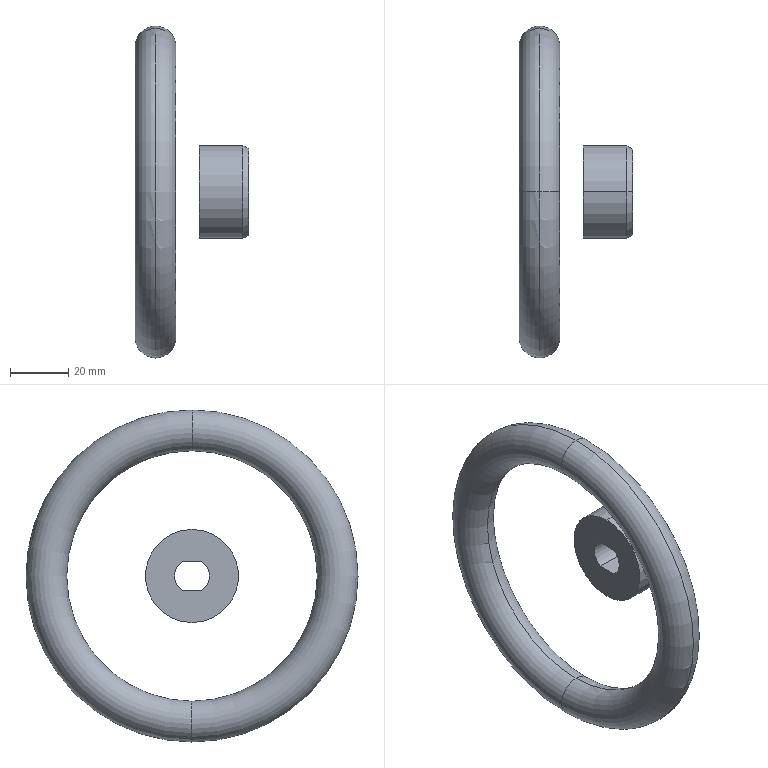Part | SolidWorks | features ICE 2, Chamfer 1, Sweep 1 | 2 solids | 14 faces | box 39 x 114 x 114 mm | volume 60150 mm3 | torus 4 | cylinder 4 | plane 4 | cone 2 | commonest cylinder face diameters 12 x2 32 x2
STEP:
#1=CARTESIAN_POINT('',(0.,-50.,-57.));
#2=VERTEX_POINT('',#1);
#3=CARTESIAN_POINT('',(0.,-50.,-43.));
#4=VERTEX_POINT('',#3);
#5=CARTESIAN_POINT('',(0.,-50.,-50.));
#6=DIRECTION('',(0.,1.,0.));
#7=DIRECTION('',(0.,0.,1.));
#8=AXIS2_PLACEMENT_3D('',#5,#6,#7);
#9=CIRCLE('',#8,7.);
#10=EDGE_CURVE('',#2,#4,#9,.T.);
#11=ORIENTED_EDGE('',*,*,#10,.F.);
#12=CARTESIAN_POINT('',(0.,-50.,57.));
#13=VERTEX_POINT('',#12);
#14=CARTESIAN_POINT('',(0.,-50.,0.));
#15=DIRECTION('',(-1.,0.,0.));
#16=DIRECTION('',(0.,0.,1.));
#17=AXIS2_PLACEMENT_3D('',#14,#15,#16);
#18=CIRCLE('',#17,57.);
#19=EDGE_CURVE('',#2,#13,#18,.T.);
#20=ORIENTED_EDGE('',*,*,#19,.T.);
#21=CARTESIAN_POINT('',(0.,-50.,43.));
#22=VERTEX_POINT('',#21);
#23=CARTESIAN_POINT('',(0.,-50.,50.));
#24=DIRECTION('',(0.,-1.,0.));
#25=DIRECTION('',(0.,0.,-1.));
#26=AXIS2_PLACEMENT_3D('',#23,#24,#25);
#27=CIRCLE('',#26,7.);
#28=EDGE_CURVE('',#13,#22,#27,.T.);
#29=ORIENTED_EDGE('',*,*,#28,.T.);
#30=CARTESIAN_POINT('',(0.,-50.,0.));
#31=DIRECTION('',(-1.,0.,0.));
#32=DIRECTION('',(0.,0.,1.));
#33=AXIS2_PLACEMENT_3D('',#30,#31,#32);
#34=CIRCLE('',#33,43.);
#35=EDGE_CURVE('',#4,#22,#34,.T.);
#36=ORIENTED_EDGE('',*,*,#35,.F.);
#37=EDGE_LOOP('',(#11,#20,#29,#36));
#38=FACE_OUTER_BOUND('',#37,.T.);
#39=CARTESIAN_POINT('',(0.,-50.,0.));
#40=DIRECTION('',(-1.,0.,0.));
#41=DIRECTION('',(0.,0.,1.));
#42=AXIS2_PLACEMENT_3D('',#39,#40,#41);
#43=TOROIDAL_SURFACE('',#42,50.,7.);
#44=ADVANCED_FACE('',(#38),#43,.T.);
#45=ORIENTED_EDGE('',*,*,#28,.F.);
#46=CARTESIAN_POINT('',(0.,-50.,0.));
#47=DIRECTION('',(-1.,0.,0.));
#48=DIRECTION('',(0.,0.,1.));
#49=AXIS2_PLACEMENT_3D('',#46,#47,#48);
#50=CIRCLE('',#49,57.);
#51=EDGE_CURVE('',#13,#2,#50,.T.);
#52=ORIENTED_EDGE('',*,*,#51,.T.);
#53=ORIENTED_EDGE('',*,*,#10,.T.);
#54=CARTESIAN_POINT('',(0.,-50.,0.));
#55=DIRECTION('',(-1.,0.,0.));
#56=DIRECTION('',(0.,0.,1.));
#57=AXIS2_PLACEMENT_3D('',#54,#55,#56);
#58=CIRCLE('',#57,43.);
#59=EDGE_CURVE('',#22,#4,#58,.T.);
#60=ORIENTED_EDGE('',*,*,#59,.F.);
#61=EDGE_LOOP('',(#45,#52,#53,#60));
#62=FACE_OUTER_BOUND('',#61,.T.);
#63=CARTESIAN_POINT('',(0.,-50.,0.));
#64=DIRECTION('',(-1.,0.,0.));
#65=DIRECTION('',(0.,0.,1.));
#66=AXIS2_PLACEMENT_3D('',#63,#64,#65);
#67=TOROIDAL_SURFACE('',#66,50.,7.);
#68=ADVANCED_FACE('',(#62),#67,.T.);
#69=ORIENTED_EDGE('',*,*,#51,.F.);
#70=CARTESIAN_POINT('',(0.,-50.,50.));
#71=DIRECTION('',(0.,-1.,0.));
#72=DIRECTION('',(0.,0.,-1.));
#73=AXIS2_PLACEMENT_3D('',#70,#71,#72);
#74=CIRCLE('',#73,7.);
#75=EDGE_CURVE('',#22,#13,#74,.T.);
#76=ORIENTED_EDGE('',*,*,#75,.F.);
#77=ORIENTED_EDGE('',*,*,#59,.T.);
#78=CARTESIAN_POINT('',(0.,-50.,-50.));
#79=DIRECTION('',(0.,1.,0.));
#80=DIRECTION('',(0.,0.,1.));
#81=AXIS2_PLACEMENT_3D('',#78,#79,#80);
#82=CIRCLE('',#81,7.);
#83=EDGE_CURVE('',#4,#2,#82,.T.);
#84=ORIENTED_EDGE('',*,*,#83,.T.);
#85=EDGE_LOOP('',(#69,#76,#77,#84));
#86=FACE_OUTER_BOUND('',#85,.T.);
#87=CARTESIAN_POINT('',(0.,-50.,0.));
#88=DIRECTION('',(-1.,0.,0.));
#89=DIRECTION('',(0.,0.,1.));
#90=AXIS2_PLACEMENT_3D('',#87,#88,#89);
#91=TOROIDAL_SURFACE('',#90,50.,7.);
#92=ADVANCED_FACE('',(#86),#91,.T.);
#93=ORIENTED_EDGE('',*,*,#19,.F.);
#94=ORIENTED_EDGE('',*,*,#83,.F.);
#95=ORIENTED_EDGE('',*,*,#35,.T.);
#96=ORIENTED_EDGE('',*,*,#75,.T.);
#97=EDGE_LOOP('',(#93,#94,#95,#96));
#98=FACE_OUTER_BOUND('',#97,.T.);
#99=CARTESIAN_POINT('',(0.,-50.,0.));
#100=DIRECTION('',(-1.,0.,0.));
#101=DIRECTION('',(0.,0.,1.));
#102=AXIS2_PLACEMENT_3D('',#99,#100,#101);
#103=TOROIDAL_SURFACE('',#102,50.,7.);
#104=ADVANCED_FACE('',(#98),#103,.T.);
#105=CLOSED_SHELL('',(#44,#68,#92,#104));
#106=MANIFOLD_SOLID_BREP('',#105);
#107=CARTESIAN_POINT('',(32.,-50.,-14.845));
#108=VERTEX_POINT('',#107);
#109=CARTESIAN_POINT('',(32.,-50.,14.845));
#110=VERTEX_POINT('',#109);
#111=CARTESIAN_POINT('',(32.,-50.,0.));
#112=DIRECTION('',(1.,0.,0.));
#113=DIRECTION('',(0.,0.,-1.));
#114=AXIS2_PLACEMENT_3D('',#111,#112,#113);
#115=CIRCLE('',#114,14.845);
#116=EDGE_CURVE('',#108,#110,#115,.T.);
#117=ORIENTED_EDGE('',*,*,#116,.F.);
#118=CARTESIAN_POINT('',(30.,-50.,-16.));
#119=VERTEX_POINT('',#118);
#120=CARTESIAN_POINT('',(32.,-50.,-14.845));
#121=DIRECTION('',(-0.866,0.,-0.5));
#122=VECTOR('',#121,1000.);
#123=LINE('',#120,#122);
#124=EDGE_CURVE('',#108,#119,#123,.T.);
#125=ORIENTED_EDGE('',*,*,#124,.T.);
#126=CARTESIAN_POINT('',(30.,-50.,16.));
#127=VERTEX_POINT('',#126);
#128=CARTESIAN_POINT('',(30.,-50.,0.));
#129=DIRECTION('',(-1.,0.,0.));
#130=DIRECTION('',(0.,0.,-1.));
#131=AXIS2_PLACEMENT_3D('',#128,#129,#130);
#132=CIRCLE('',#131,16.);
#133=EDGE_CURVE('',#127,#119,#132,.T.);
#134=ORIENTED_EDGE('',*,*,#133,.F.);
#135=CARTESIAN_POINT('',(32.,-50.,14.845));
#136=DIRECTION('',(-0.866,0.,0.5));
#137=VECTOR('',#136,1000.);
#138=LINE('',#135,#137);
#139=EDGE_CURVE('',#110,#127,#138,.T.);
#140=ORIENTED_EDGE('',*,*,#139,.F.);
#141=EDGE_LOOP('',(#117,#125,#134,#140));
#142=FACE_OUTER_BOUND('',#141,.T.);
#143=CARTESIAN_POINT('',(32.,-50.,0.));
#144=DIRECTION('',(-1.,0.,0.));
#145=DIRECTION('',(0.,0.,1.));
#146=AXIS2_PLACEMENT_3D('',#143,#144,#145);
#147=CONICAL_SURFACE('',#146,14.845,0.5236);
#148=ADVANCED_FACE('',(#142),#147,.T.);
#149=CARTESIAN_POINT('',(15.,-50.,-16.));
#150=VERTEX_POINT('',#149);
#151=CARTESIAN_POINT('',(15.,-50.,16.));
#152=VERTEX_POINT('',#151);
#153=CARTESIAN_POINT('',(15.,-50.,0.));
#154=DIRECTION('',(1.,0.,0.));
#155=DIRECTION('',(0.,0.,-1.));
#156=AXIS2_PLACEMENT_3D('',#153,#154,#155);
#157=CIRCLE('',#156,16.);
#158=EDGE_CURVE('',#150,#152,#157,.T.);
#159=ORIENTED_EDGE('',*,*,#158,.T.);
#160=CARTESIAN_POINT('',(15.,-50.,16.));
#161=DIRECTION('',(1.,0.,0.));
#162=VECTOR('',#161,1000.);
#163=LINE('',#160,#162);
#164=EDGE_CURVE('',#152,#127,#163,.T.);
#165=ORIENTED_EDGE('',*,*,#164,.T.);
#166=ORIENTED_EDGE('',*,*,#133,.T.);
#167=CARTESIAN_POINT('',(15.,-50.,-16.));
#168=DIRECTION('',(1.,0.,0.));
#169=VECTOR('',#168,1000.);
#170=LINE('',#167,#169);
#171=EDGE_CURVE('',#150,#119,#170,.T.);
#172=ORIENTED_EDGE('',*,*,#171,.F.);
#173=EDGE_LOOP('',(#159,#165,#166,#172));
#174=FACE_OUTER_BOUND('',#173,.T.);
#175=CARTESIAN_POINT('',(15.,-50.,0.));
#176=DIRECTION('',(1.,0.,0.));
#177=DIRECTION('',(0.,0.,-1.));
#178=AXIS2_PLACEMENT_3D('',#175,#176,#177);
#179=CYLINDRICAL_SURFACE('',#178,16.);
#180=ADVANCED_FACE('',(#174),#179,.T.);
#181=ORIENTED_EDGE('',*,*,#164,.F.);
#182=CARTESIAN_POINT('',(15.,-50.,0.));
#183=DIRECTION('',(1.,0.,0.));
#184=DIRECTION('',(0.,0.,-1.));
#185=AXIS2_PLACEMENT_3D('',#182,#183,#184);
#186=CIRCLE('',#185,16.);
#187=EDGE_CURVE('',#152,#150,#186,.T.);
#188=ORIENTED_EDGE('',*,*,#187,.T.);
#189=ORIENTED_EDGE('',*,*,#171,.T.);
#190=CARTESIAN_POINT('',(30.,-50.,0.));
#191=DIRECTION('',(-1.,0.,0.));
#192=DIRECTION('',(0.,0.,-1.));
#193=AXIS2_PLACEMENT_3D('',#190,#191,#192);
#194=CIRCLE('',#193,16.);
#195=EDGE_CURVE('',#119,#127,#194,.T.);
#196=ORIENTED_EDGE('',*,*,#195,.T.);
#197=EDGE_LOOP('',(#181,#188,#189,#196));
#198=FACE_OUTER_BOUND('',#197,.T.);
#199=CARTESIAN_POINT('',(15.,-50.,0.));
#200=DIRECTION('',(1.,0.,0.));
#201=DIRECTION('',(0.,0.,-1.));
#202=AXIS2_PLACEMENT_3D('',#199,#200,#201);
#203=CYLINDRICAL_SURFACE('',#202,16.);
#204=ADVANCED_FACE('',(#198),#203,.T.);
#205=CARTESIAN_POINT('',(15.,-53.317,-5.));
#206=VERTEX_POINT('',#205);
#207=CARTESIAN_POINT('',(15.,-46.683,-5.));
#208=VERTEX_POINT('',#207);
#209=CARTESIAN_POINT('',(15.,-50.,-5.));
#210=DIRECTION('',(0.,1.,0.));
#211=VECTOR('',#210,1000.);
#212=LINE('',#209,#211);
#213=EDGE_CURVE('',#206,#208,#212,.T.);
#214=ORIENTED_EDGE('',*,*,#213,.T.);
#215=CARTESIAN_POINT('',(15.,-46.683,5.));
#216=VERTEX_POINT('',#215);
#217=CARTESIAN_POINT('',(15.,-50.,0.));
#218=DIRECTION('',(1.,0.,0.));
#219=DIRECTION('',(0.,0.,-1.));
#220=AXIS2_PLACEMENT_3D('',#217,#218,#219);
#221=CIRCLE('',#220,6.);
#222=EDGE_CURVE('',#208,#216,#221,.T.);
#223=ORIENTED_EDGE('',*,*,#222,.T.);
#224=CARTESIAN_POINT('',(15.,-53.317,5.));
#225=VERTEX_POINT('',#224);
#226=CARTESIAN_POINT('',(15.,-50.,5.));
#227=DIRECTION('',(0.,-1.,0.));
#228=VECTOR('',#227,1000.);
#229=LINE('',#226,#228);
#230=EDGE_CURVE('',#216,#225,#229,.T.);
#231=ORIENTED_EDGE('',*,*,#230,.T.);
#232=CARTESIAN_POINT('',(15.,-50.,0.));
#233=DIRECTION('',(1.,0.,0.));
#234=DIRECTION('',(0.,0.,-1.));
#235=AXIS2_PLACEMENT_3D('',#232,#233,#234);
#236=CIRCLE('',#235,6.);
#237=EDGE_CURVE('',#225,#206,#236,.T.);
#238=ORIENTED_EDGE('',*,*,#237,.T.);
#239=EDGE_LOOP('',(#214,#223,#231,#238));
#240=FACE_BOUND('',#239,.T.);
#241=ORIENTED_EDGE('',*,*,#158,.F.);
#242=ORIENTED_EDGE('',*,*,#187,.F.);
#243=EDGE_LOOP('',(#241,#242));
#244=FACE_OUTER_BOUND('',#243,.T.);
#245=CARTESIAN_POINT('',(15.,-50.,0.));
#246=DIRECTION('',(1.,0.,0.));
#247=DIRECTION('',(0.,0.,-1.));
#248=AXIS2_PLACEMENT_3D('',#245,#246,#247);
#249=PLANE('',#248);
#250=ADVANCED_FACE('',(#240,#244),#249,.F.);
#251=CARTESIAN_POINT('',(32.,-46.683,-5.));
#252=VERTEX_POINT('',#251);
#253=CARTESIAN_POINT('',(32.,-46.683,5.));
#254=VERTEX_POINT('',#253);
#255=CARTESIAN_POINT('',(32.,-50.,0.));
#256=DIRECTION('',(1.,0.,0.));
#257=DIRECTION('',(0.,0.,-1.));
#258=AXIS2_PLACEMENT_3D('',#255,#256,#257);
#259=CIRCLE('',#258,6.);
#260=EDGE_CURVE('',#252,#254,#259,.T.);
#261=ORIENTED_EDGE('',*,*,#260,.F.);
#262=CARTESIAN_POINT('',(32.,-53.317,-5.));
#263=VERTEX_POINT('',#262);
#264=CARTESIAN_POINT('',(32.,-46.683,-5.));
#265=DIRECTION('',(0.,1.,0.));
#266=VECTOR('',#265,1000.);
#267=LINE('',#264,#266);
#268=EDGE_CURVE('',#263,#252,#267,.T.);
#269=ORIENTED_EDGE('',*,*,#268,.F.);
#270=CARTESIAN_POINT('',(32.,-53.317,5.));
#271=VERTEX_POINT('',#270);
#272=CARTESIAN_POINT('',(32.,-50.,0.));
#273=DIRECTION('',(1.,0.,0.));
#274=DIRECTION('',(0.,0.,-1.));
#275=AXIS2_PLACEMENT_3D('',#272,#273,#274);
#276=CIRCLE('',#275,6.);
#277=EDGE_CURVE('',#271,#263,#276,.T.);
#278=ORIENTED_EDGE('',*,*,#277,.F.);
#279=CARTESIAN_POINT('',(32.,-46.683,5.));
#280=DIRECTION('',(0.,-1.,0.));
#281=VECTOR('',#280,1000.);
#282=LINE('',#279,#281);
#283=EDGE_CURVE('',#254,#271,#282,.T.);
#284=ORIENTED_EDGE('',*,*,#283,.F.);
#285=EDGE_LOOP('',(#261,#269,#278,#284));
#286=FACE_BOUND('',#285,.T.);
#287=CARTESIAN_POINT('',(32.,-50.,0.));
#288=DIRECTION('',(1.,0.,0.));
#289=DIRECTION('',(0.,0.,-1.));
#290=AXIS2_PLACEMENT_3D('',#287,#288,#289);
#291=CIRCLE('',#290,14.845);
#292=EDGE_CURVE('',#110,#108,#291,.T.);
#293=ORIENTED_EDGE('',*,*,#292,.T.);
#294=ORIENTED_EDGE('',*,*,#116,.T.);
#295=EDGE_LOOP('',(#293,#294));
#296=FACE_OUTER_BOUND('',#295,.T.);
#297=CARTESIAN_POINT('',(32.,-50.,0.));
#298=DIRECTION('',(1.,0.,0.));
#299=DIRECTION('',(0.,0.,-1.));
#300=AXIS2_PLACEMENT_3D('',#297,#298,#299);
#301=PLANE('',#300);
#302=ADVANCED_FACE('',(#286,#296),#301,.T.);
#303=ORIENTED_EDGE('',*,*,#124,.F.);
#304=ORIENTED_EDGE('',*,*,#292,.F.);
#305=ORIENTED_EDGE('',*,*,#139,.T.);
#306=ORIENTED_EDGE('',*,*,#195,.F.);
#307=EDGE_LOOP('',(#303,#304,#305,#306));
#308=FACE_OUTER_BOUND('',#307,.T.);
#309=CARTESIAN_POINT('',(32.,-50.,0.));
#310=DIRECTION('',(-1.,0.,0.));
#311=DIRECTION('',(0.,0.,1.));
#312=AXIS2_PLACEMENT_3D('',#309,#310,#311);
#313=CONICAL_SURFACE('',#312,14.845,0.5236);
#314=ADVANCED_FACE('',(#308),#313,.T.);
#315=CARTESIAN_POINT('',(-7.,-46.683,-5.));
#316=DIRECTION('',(1.,0.,0.));
#317=VECTOR('',#316,1000.);
#318=LINE('',#315,#317);
#319=EDGE_CURVE('',#208,#252,#318,.T.);
#320=ORIENTED_EDGE('',*,*,#319,.T.);
#321=ORIENTED_EDGE('',*,*,#260,.T.);
#322=CARTESIAN_POINT('',(-7.,-46.683,5.));
#323=DIRECTION('',(1.,0.,0.));
#324=VECTOR('',#323,1000.);
#325=LINE('',#322,#324);
#326=EDGE_CURVE('',#216,#254,#325,.T.);
#327=ORIENTED_EDGE('',*,*,#326,.F.);
#328=ORIENTED_EDGE('',*,*,#222,.F.);
#329=EDGE_LOOP('',(#320,#321,#327,#328));
#330=FACE_OUTER_BOUND('',#329,.T.);
#331=CARTESIAN_POINT('',(-7.,-50.,0.));
#332=DIRECTION('',(1.,0.,0.));
#333=DIRECTION('',(0.,0.,-1.));
#334=AXIS2_PLACEMENT_3D('',#331,#332,#333);
#335=CYLINDRICAL_SURFACE('',#334,6.);
#336=ADVANCED_FACE('',(#330),#335,.F.);
#337=CARTESIAN_POINT('',(-7.,-53.317,-5.));
#338=DIRECTION('',(1.,0.,0.));
#339=VECTOR('',#338,1000.);
#340=LINE('',#337,#339);
#341=EDGE_CURVE('',#206,#263,#340,.T.);
#342=ORIENTED_EDGE('',*,*,#341,.T.);
#343=ORIENTED_EDGE('',*,*,#268,.T.);
#344=ORIENTED_EDGE('',*,*,#319,.F.);
#345=ORIENTED_EDGE('',*,*,#213,.F.);
#346=EDGE_LOOP('',(#342,#343,#344,#345));
#347=FACE_OUTER_BOUND('',#346,.T.);
#348=CARTESIAN_POINT('',(-7.,-46.683,-5.));
#349=DIRECTION('',(0.,0.,-1.));
#350=DIRECTION('',(-1.,0.,0.));
#351=AXIS2_PLACEMENT_3D('',#348,#349,#350);
#352=PLANE('',#351);
#353=ADVANCED_FACE('',(#347),#352,.F.);
#354=CARTESIAN_POINT('',(-7.,-53.317,5.));
#355=DIRECTION('',(1.,0.,0.));
#356=VECTOR('',#355,1000.);
#357=LINE('',#354,#356);
#358=EDGE_CURVE('',#225,#271,#357,.T.);
#359=ORIENTED_EDGE('',*,*,#358,.T.);
#360=ORIENTED_EDGE('',*,*,#277,.T.);
#361=ORIENTED_EDGE('',*,*,#341,.F.);
#362=ORIENTED_EDGE('',*,*,#237,.F.);
#363=EDGE_LOOP('',(#359,#360,#361,#362));
#364=FACE_OUTER_BOUND('',#363,.T.);
#365=CARTESIAN_POINT('',(-7.,-50.,0.));
#366=DIRECTION('',(1.,0.,0.));
#367=DIRECTION('',(0.,0.,-1.));
#368=AXIS2_PLACEMENT_3D('',#365,#366,#367);
#369=CYLINDRICAL_SURFACE('',#368,6.);
#370=ADVANCED_FACE('',(#364),#369,.F.);
#371=ORIENTED_EDGE('',*,*,#326,.T.);
#372=ORIENTED_EDGE('',*,*,#283,.T.);
#373=ORIENTED_EDGE('',*,*,#358,.F.);
#374=ORIENTED_EDGE('',*,*,#230,.F.);
#375=EDGE_LOOP('',(#371,#372,#373,#374));
#376=FACE_OUTER_BOUND('',#375,.T.);
#377=CARTESIAN_POINT('',(-7.,-46.683,5.));
#378=DIRECTION('',(0.,0.,1.));
#379=DIRECTION('',(1.,0.,0.));
#380=AXIS2_PLACEMENT_3D('',#377,#378,#379);
#381=PLANE('',#380);
#382=ADVANCED_FACE('',(#376),#381,.F.);
#383=CLOSED_SHELL('',(#148,#180,#204,#250,#302,#314,#336,#353,#370,#382));
#384=MANIFOLD_SOLID_BREP('',#383);
#385=CARTESIAN_POINT('',(0.,0.,0.));
#386=DIRECTION('',(0.,0.,1.));
#387=DIRECTION('',(1.,0.,0.));
#388=AXIS2_PLACEMENT_3D('',#385,#386,#387);
#389=(LENGTH_UNIT()NAMED_UNIT(*)SI_UNIT(.MILLI.,.METRE.));
#390=UNCERTAINTY_MEASURE_WITH_UNIT(LENGTH_MEASURE(0.00001),#389,'','');
#391=(NAMED_UNIT(*)PLANE_ANGLE_UNIT()SI_UNIT($,.RADIAN.));
#392=(NAMED_UNIT(*)SI_UNIT($,.STERADIAN.)SOLID_ANGLE_UNIT());
#393=(GEOMETRIC_REPRESENTATION_CONTEXT(3)GLOBAL_UNCERTAINTY_ASSIGNED_CONTEXT((#390))GLOBAL_UNIT_ASSIGNED_CONTEXT((#389,#391,#392))REPRESENTATION_CONTEXT('',''));
#394=ADVANCED_BREP_SHAPE_REPRESENTATION('',(#106,#384,#388),#393);